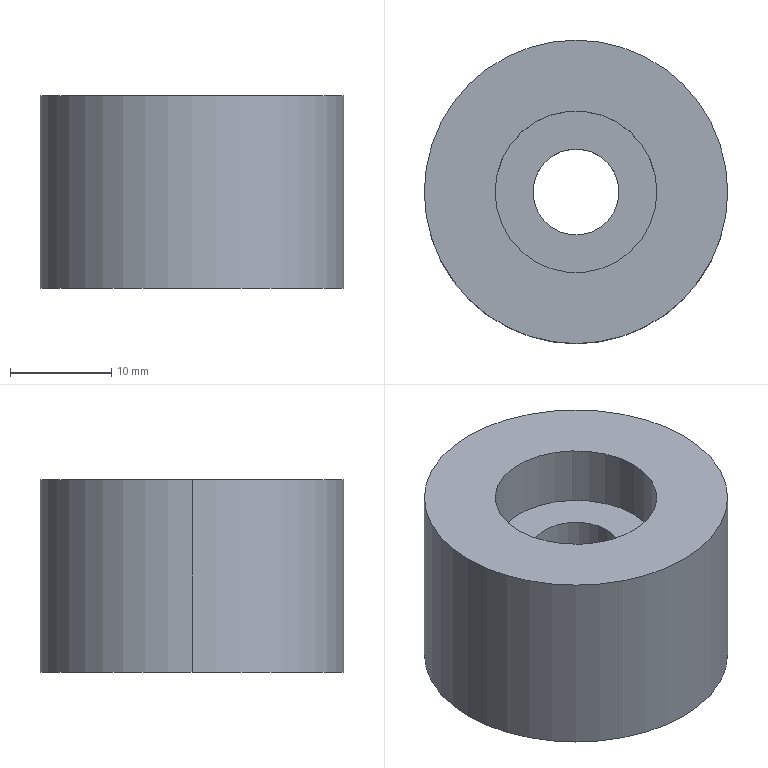Part | STEP file | POM limit 1 | 1 solid | 9 faces | box 30 x 30 x 19 mm | volume 11486 mm3 | cylinder 6 | plane 3 | commonest cylinder face diameters 8.5 x2 16 x2 30 x2
STEP:
#1=CARTESIAN_POINT('',(0.,0.,0.));
#2=DIRECTION('',(0.,0.,1.));
#3=DIRECTION('',(1.,0.,0.));
#4=AXIS2_PLACEMENT_3D('',#1,#2,#3);
#5=CARTESIAN_POINT('',(8.,0.,13.));
#6=VERTEX_POINT('',#5);
#7=CARTESIAN_POINT('',(8.,0.,19.));
#8=VERTEX_POINT('',#7);
#9=CARTESIAN_POINT('',(8.,0.,13.));
#10=DIRECTION('',(0.,0.,1.));
#11=VECTOR('',#10,1.);
#12=LINE('',#9,#11);
#13=CARTESIAN_POINT('',(0.,0.,13.));
#14=DIRECTION('',(0.,0.,1.));
#15=DIRECTION('',(1.,0.,0.));
#16=AXIS2_PLACEMENT_3D('',#13,#14,#15);
#17=CYLINDRICAL_SURFACE('',#16,8.);
#18=CARTESIAN_POINT('',(6.283,0.));
#19=DIRECTION('',(0.,1.));
#20=VECTOR('',#19,1.);
#21=LINE('',#18,#20);
#22=(GEOMETRIC_REPRESENTATION_CONTEXT(2)PARAMETRIC_REPRESENTATION_CONTEXT()REPRESENTATION_CONTEXT('',''));
#23=DEFINITIONAL_REPRESENTATION('',(#21),#22);
#24=PCURVE('',#17,#23);
#25=CARTESIAN_POINT('',(0.,0.,13.));
#26=DIRECTION('',(0.,0.,1.));
#27=DIRECTION('',(1.,0.,0.));
#28=AXIS2_PLACEMENT_3D('',#25,#26,#27);
#29=CYLINDRICAL_SURFACE('',#28,8.);
#30=CARTESIAN_POINT('',(0.,0.));
#31=DIRECTION('',(0.,1.));
#32=VECTOR('',#31,1.);
#33=LINE('',#30,#32);
#34=(GEOMETRIC_REPRESENTATION_CONTEXT(2)PARAMETRIC_REPRESENTATION_CONTEXT()REPRESENTATION_CONTEXT('',''));
#35=DEFINITIONAL_REPRESENTATION('',(#33),#34);
#36=PCURVE('',#29,#35);
#37=SURFACE_CURVE('',#12,(#24,#36),.PCURVE_S1.);
#38=EDGE_CURVE('',#6,#8,#37,.T.);
#39=ORIENTED_EDGE('',*,*,#38,.T.);
#40=CARTESIAN_POINT('',(-8.,0.,19.));
#41=VERTEX_POINT('',#40);
#42=CARTESIAN_POINT('',(0.,0.,19.));
#43=DIRECTION('',(0.,0.,1.));
#44=DIRECTION('',(1.,0.,0.));
#45=AXIS2_PLACEMENT_3D('',#42,#43,#44);
#46=CIRCLE('',#45,8.);
#47=CARTESIAN_POINT('',(0.,6.));
#48=DIRECTION('',(1.,0.));
#49=VECTOR('',#48,1.);
#50=LINE('',#47,#49);
#51=(GEOMETRIC_REPRESENTATION_CONTEXT(2)PARAMETRIC_REPRESENTATION_CONTEXT()REPRESENTATION_CONTEXT('',''));
#52=DEFINITIONAL_REPRESENTATION('',(#50),#51);
#53=PCURVE('',#17,#52);
#54=CARTESIAN_POINT('',(0.,0.,19.));
#55=DIRECTION('',(0.,0.,1.));
#56=DIRECTION('',(1.,0.,0.));
#57=AXIS2_PLACEMENT_3D('',#54,#55,#56);
#58=PLANE('',#57);
#59=CARTESIAN_POINT('',(0.,0.));
#60=DIRECTION('',(1.,0.));
#61=AXIS2_PLACEMENT_2D('',#59,#60);
#62=CIRCLE('',#61,8.);
#63=(GEOMETRIC_REPRESENTATION_CONTEXT(2)PARAMETRIC_REPRESENTATION_CONTEXT()REPRESENTATION_CONTEXT('',''));
#64=DEFINITIONAL_REPRESENTATION('',(#62),#63);
#65=PCURVE('',#58,#64);
#66=SURFACE_CURVE('',#46,(#53,#65),.PCURVE_S1.);
#67=EDGE_CURVE('',#41,#8,#66,.T.);
#68=ORIENTED_EDGE('',*,*,#67,.F.);
#69=CARTESIAN_POINT('',(-8.,0.,13.));
#70=VERTEX_POINT('',#69);
#71=CARTESIAN_POINT('',(-8.,0.,13.));
#72=DIRECTION('',(0.,0.,1.));
#73=VECTOR('',#72,1.);
#74=LINE('',#71,#73);
#75=CARTESIAN_POINT('',(3.142,0.));
#76=DIRECTION('',(0.,1.));
#77=VECTOR('',#76,1.);
#78=LINE('',#75,#77);
#79=(GEOMETRIC_REPRESENTATION_CONTEXT(2)PARAMETRIC_REPRESENTATION_CONTEXT()REPRESENTATION_CONTEXT('',''));
#80=DEFINITIONAL_REPRESENTATION('',(#78),#79);
#81=PCURVE('',#17,#80);
#82=CARTESIAN_POINT('',(3.142,0.));
#83=DIRECTION('',(0.,1.));
#84=VECTOR('',#83,1.);
#85=LINE('',#82,#84);
#86=(GEOMETRIC_REPRESENTATION_CONTEXT(2)PARAMETRIC_REPRESENTATION_CONTEXT()REPRESENTATION_CONTEXT('',''));
#87=DEFINITIONAL_REPRESENTATION('',(#85),#86);
#88=PCURVE('',#29,#87);
#89=SURFACE_CURVE('',#74,(#81,#88),.PCURVE_S1.);
#90=EDGE_CURVE('',#70,#41,#89,.T.);
#91=ORIENTED_EDGE('',*,*,#90,.F.);
#92=CARTESIAN_POINT('',(0.,0.,13.));
#93=DIRECTION('',(0.,0.,1.));
#94=DIRECTION('',(1.,0.,0.));
#95=AXIS2_PLACEMENT_3D('',#92,#93,#94);
#96=CIRCLE('',#95,8.);
#97=CARTESIAN_POINT('',(0.,0.));
#98=DIRECTION('',(1.,0.));
#99=VECTOR('',#98,1.);
#100=LINE('',#97,#99);
#101=(GEOMETRIC_REPRESENTATION_CONTEXT(2)PARAMETRIC_REPRESENTATION_CONTEXT()REPRESENTATION_CONTEXT('',''));
#102=DEFINITIONAL_REPRESENTATION('',(#100),#101);
#103=PCURVE('',#17,#102);
#104=CARTESIAN_POINT('',(0.,0.,13.));
#105=DIRECTION('',(0.,0.,1.));
#106=DIRECTION('',(1.,0.,0.));
#107=AXIS2_PLACEMENT_3D('',#104,#105,#106);
#108=PLANE('',#107);
#109=CARTESIAN_POINT('',(0.,0.));
#110=DIRECTION('',(1.,0.));
#111=AXIS2_PLACEMENT_2D('',#109,#110);
#112=CIRCLE('',#111,8.);
#113=(GEOMETRIC_REPRESENTATION_CONTEXT(2)PARAMETRIC_REPRESENTATION_CONTEXT()REPRESENTATION_CONTEXT('',''));
#114=DEFINITIONAL_REPRESENTATION('',(#112),#113);
#115=PCURVE('',#108,#114);
#116=SURFACE_CURVE('',#96,(#103,#115),.PCURVE_S1.);
#117=EDGE_CURVE('',#70,#6,#116,.T.);
#118=ORIENTED_EDGE('',*,*,#117,.T.);
#119=EDGE_LOOP('',(#39,#68,#91,#118));
#120=FACE_BOUND('',#119,.F.);
#121=ADVANCED_FACE('',(#120),#17,.F.);
#122=CARTESIAN_POINT('',(15.,0.,19.));
#123=VERTEX_POINT('',#122);
#124=CARTESIAN_POINT('',(-15.,0.,19.));
#125=VERTEX_POINT('',#124);
#126=CARTESIAN_POINT('',(0.,0.,19.));
#127=DIRECTION('',(0.,0.,1.));
#128=DIRECTION('',(1.,0.,0.));
#129=AXIS2_PLACEMENT_3D('',#126,#127,#128);
#130=CIRCLE('',#129,15.);
#131=CARTESIAN_POINT('',(0.,0.,19.));
#132=DIRECTION('',(0.,0.,-1.));
#133=DIRECTION('',(-1.,0.,0.));
#134=AXIS2_PLACEMENT_3D('',#131,#132,#133);
#135=CYLINDRICAL_SURFACE('',#134,15.);
#136=CARTESIAN_POINT('',(3.142,0.));
#137=DIRECTION('',(-1.,0.));
#138=VECTOR('',#137,1.);
#139=LINE('',#136,#138);
#140=(GEOMETRIC_REPRESENTATION_CONTEXT(2)PARAMETRIC_REPRESENTATION_CONTEXT()REPRESENTATION_CONTEXT('',''));
#141=DEFINITIONAL_REPRESENTATION('',(#139),#140);
#142=PCURVE('',#135,#141);
#143=CARTESIAN_POINT('',(0.,0.));
#144=DIRECTION('',(1.,0.));
#145=AXIS2_PLACEMENT_2D('',#143,#144);
#146=CIRCLE('',#145,15.);
#147=(GEOMETRIC_REPRESENTATION_CONTEXT(2)PARAMETRIC_REPRESENTATION_CONTEXT()REPRESENTATION_CONTEXT('',''));
#148=DEFINITIONAL_REPRESENTATION('',(#146),#147);
#149=PCURVE('',#58,#148);
#150=SURFACE_CURVE('',#130,(#142,#149),.PCURVE_S1.);
#151=EDGE_CURVE('',#123,#125,#150,.T.);
#152=ORIENTED_EDGE('',*,*,#151,.F.);
#153=CARTESIAN_POINT('',(15.,0.,0.));
#154=VERTEX_POINT('',#153);
#155=CARTESIAN_POINT('',(15.,0.,19.));
#156=DIRECTION('',(0.,0.,-1.));
#157=VECTOR('',#156,1.);
#158=LINE('',#155,#157);
#159=CARTESIAN_POINT('',(3.142,0.));
#160=DIRECTION('',(0.,1.));
#161=VECTOR('',#160,1.);
#162=LINE('',#159,#161);
#163=(GEOMETRIC_REPRESENTATION_CONTEXT(2)PARAMETRIC_REPRESENTATION_CONTEXT()REPRESENTATION_CONTEXT('',''));
#164=DEFINITIONAL_REPRESENTATION('',(#162),#163);
#165=PCURVE('',#135,#164);
#166=CARTESIAN_POINT('',(0.,0.,19.));
#167=DIRECTION('',(0.,0.,-1.));
#168=DIRECTION('',(-1.,0.,0.));
#169=AXIS2_PLACEMENT_3D('',#166,#167,#168);
#170=CYLINDRICAL_SURFACE('',#169,15.);
#171=CARTESIAN_POINT('',(3.142,0.));
#172=DIRECTION('',(0.,1.));
#173=VECTOR('',#172,1.);
#174=LINE('',#171,#173);
#175=(GEOMETRIC_REPRESENTATION_CONTEXT(2)PARAMETRIC_REPRESENTATION_CONTEXT()REPRESENTATION_CONTEXT('',''));
#176=DEFINITIONAL_REPRESENTATION('',(#174),#175);
#177=PCURVE('',#170,#176);
#178=SURFACE_CURVE('',#158,(#165,#177),.PCURVE_S1.);
#179=EDGE_CURVE('',#123,#154,#178,.T.);
#180=ORIENTED_EDGE('',*,*,#179,.T.);
#181=CARTESIAN_POINT('',(-15.,0.,0.));
#182=VERTEX_POINT('',#181);
#183=CARTESIAN_POINT('',(0.,0.,0.));
#184=DIRECTION('',(0.,0.,1.));
#185=DIRECTION('',(1.,0.,0.));
#186=AXIS2_PLACEMENT_3D('',#183,#184,#185);
#187=CIRCLE('',#186,15.);
#188=CARTESIAN_POINT('',(3.142,19.));
#189=DIRECTION('',(-1.,0.));
#190=VECTOR('',#189,1.);
#191=LINE('',#188,#190);
#192=(GEOMETRIC_REPRESENTATION_CONTEXT(2)PARAMETRIC_REPRESENTATION_CONTEXT()REPRESENTATION_CONTEXT('',''));
#193=DEFINITIONAL_REPRESENTATION('',(#191),#192);
#194=PCURVE('',#135,#193);
#195=CARTESIAN_POINT('',(0.,0.,0.));
#196=DIRECTION('',(0.,0.,1.));
#197=DIRECTION('',(1.,0.,0.));
#198=AXIS2_PLACEMENT_3D('',#195,#196,#197);
#199=PLANE('',#198);
#200=CARTESIAN_POINT('',(0.,0.));
#201=DIRECTION('',(1.,0.));
#202=AXIS2_PLACEMENT_2D('',#200,#201);
#203=CIRCLE('',#202,15.);
#204=(GEOMETRIC_REPRESENTATION_CONTEXT(2)PARAMETRIC_REPRESENTATION_CONTEXT()REPRESENTATION_CONTEXT('',''));
#205=DEFINITIONAL_REPRESENTATION('',(#203),#204);
#206=PCURVE('',#199,#205);
#207=SURFACE_CURVE('',#187,(#194,#206),.PCURVE_S1.);
#208=EDGE_CURVE('',#154,#182,#207,.T.);
#209=ORIENTED_EDGE('',*,*,#208,.T.);
#210=CARTESIAN_POINT('',(-15.,0.,19.));
#211=DIRECTION('',(0.,0.,-1.));
#212=VECTOR('',#211,1.);
#213=LINE('',#210,#212);
#214=CARTESIAN_POINT('',(0.,0.));
#215=DIRECTION('',(0.,1.));
#216=VECTOR('',#215,1.);
#217=LINE('',#214,#216);
#218=(GEOMETRIC_REPRESENTATION_CONTEXT(2)PARAMETRIC_REPRESENTATION_CONTEXT()REPRESENTATION_CONTEXT('',''));
#219=DEFINITIONAL_REPRESENTATION('',(#217),#218);
#220=PCURVE('',#135,#219);
#221=CARTESIAN_POINT('',(6.283,0.));
#222=DIRECTION('',(0.,1.));
#223=VECTOR('',#222,1.);
#224=LINE('',#221,#223);
#225=(GEOMETRIC_REPRESENTATION_CONTEXT(2)PARAMETRIC_REPRESENTATION_CONTEXT()REPRESENTATION_CONTEXT('',''));
#226=DEFINITIONAL_REPRESENTATION('',(#224),#225);
#227=PCURVE('',#170,#226);
#228=SURFACE_CURVE('',#213,(#220,#227),.PCURVE_S1.);
#229=EDGE_CURVE('',#125,#182,#228,.T.);
#230=ORIENTED_EDGE('',*,*,#229,.F.);
#231=EDGE_LOOP('',(#152,#180,#209,#230));
#232=FACE_BOUND('',#231,.T.);
#233=ADVANCED_FACE('',(#232),#135,.T.);
#234=CARTESIAN_POINT('',(-4.25,0.,13.));
#235=VERTEX_POINT('',#234);
#236=CARTESIAN_POINT('',(-4.25,0.,0.));
#237=VERTEX_POINT('',#236);
#238=CARTESIAN_POINT('',(-4.25,0.,19.));
#239=DIRECTION('',(0.,0.,-1.));
#240=VECTOR('',#239,1.);
#241=LINE('',#238,#240);
#242=CARTESIAN_POINT('',(0.,0.,19.));
#243=DIRECTION('',(0.,0.,-1.));
#244=DIRECTION('',(-1.,0.,0.));
#245=AXIS2_PLACEMENT_3D('',#242,#243,#244);
#246=CYLINDRICAL_SURFACE('',#245,4.25);
#247=CARTESIAN_POINT('',(6.283,0.));
#248=DIRECTION('',(0.,1.));
#249=VECTOR('',#248,1.);
#250=LINE('',#247,#249);
#251=(GEOMETRIC_REPRESENTATION_CONTEXT(2)PARAMETRIC_REPRESENTATION_CONTEXT()REPRESENTATION_CONTEXT('',''));
#252=DEFINITIONAL_REPRESENTATION('',(#250),#251);
#253=PCURVE('',#246,#252);
#254=CARTESIAN_POINT('',(0.,0.,19.));
#255=DIRECTION('',(0.,0.,-1.));
#256=DIRECTION('',(-1.,0.,0.));
#257=AXIS2_PLACEMENT_3D('',#254,#255,#256);
#258=CYLINDRICAL_SURFACE('',#257,4.25);
#259=CARTESIAN_POINT('',(0.,0.));
#260=DIRECTION('',(0.,1.));
#261=VECTOR('',#260,1.);
#262=LINE('',#259,#261);
#263=(GEOMETRIC_REPRESENTATION_CONTEXT(2)PARAMETRIC_REPRESENTATION_CONTEXT()REPRESENTATION_CONTEXT('',''));
#264=DEFINITIONAL_REPRESENTATION('',(#262),#263);
#265=PCURVE('',#258,#264);
#266=SURFACE_CURVE('',#241,(#253,#265),.PCURVE_S1.);
#267=EDGE_CURVE('',#235,#237,#266,.T.);
#268=ORIENTED_EDGE('',*,*,#267,.T.);
#269=CARTESIAN_POINT('',(4.25,0.,0.));
#270=VERTEX_POINT('',#269);
#271=CARTESIAN_POINT('',(0.,0.,0.));
#272=DIRECTION('',(0.,0.,1.));
#273=DIRECTION('',(1.,0.,0.));
#274=AXIS2_PLACEMENT_3D('',#271,#272,#273);
#275=CIRCLE('',#274,4.25);
#276=CARTESIAN_POINT('',(9.425,19.));
#277=DIRECTION('',(-1.,0.));
#278=VECTOR('',#277,1.);
#279=LINE('',#276,#278);
#280=(GEOMETRIC_REPRESENTATION_CONTEXT(2)PARAMETRIC_REPRESENTATION_CONTEXT()REPRESENTATION_CONTEXT('',''));
#281=DEFINITIONAL_REPRESENTATION('',(#279),#280);
#282=PCURVE('',#246,#281);
#283=CARTESIAN_POINT('',(0.,0.));
#284=DIRECTION('',(1.,0.));
#285=AXIS2_PLACEMENT_2D('',#283,#284);
#286=CIRCLE('',#285,4.25);
#287=(GEOMETRIC_REPRESENTATION_CONTEXT(2)PARAMETRIC_REPRESENTATION_CONTEXT()REPRESENTATION_CONTEXT('',''));
#288=DEFINITIONAL_REPRESENTATION('',(#286),#287);
#289=PCURVE('',#199,#288);
#290=SURFACE_CURVE('',#275,(#282,#289),.PCURVE_S1.);
#291=EDGE_CURVE('',#237,#270,#290,.T.);
#292=ORIENTED_EDGE('',*,*,#291,.T.);
#293=CARTESIAN_POINT('',(4.25,0.,13.));
#294=VERTEX_POINT('',#293);
#295=CARTESIAN_POINT('',(4.25,0.,19.));
#296=DIRECTION('',(0.,0.,-1.));
#297=VECTOR('',#296,1.);
#298=LINE('',#295,#297);
#299=CARTESIAN_POINT('',(3.142,0.));
#300=DIRECTION('',(0.,1.));
#301=VECTOR('',#300,1.);
#302=LINE('',#299,#301);
#303=(GEOMETRIC_REPRESENTATION_CONTEXT(2)PARAMETRIC_REPRESENTATION_CONTEXT()REPRESENTATION_CONTEXT('',''));
#304=DEFINITIONAL_REPRESENTATION('',(#302),#303);
#305=PCURVE('',#246,#304);
#306=CARTESIAN_POINT('',(3.142,0.));
#307=DIRECTION('',(0.,1.));
#308=VECTOR('',#307,1.);
#309=LINE('',#306,#308);
#310=(GEOMETRIC_REPRESENTATION_CONTEXT(2)PARAMETRIC_REPRESENTATION_CONTEXT()REPRESENTATION_CONTEXT('',''));
#311=DEFINITIONAL_REPRESENTATION('',(#309),#310);
#312=PCURVE('',#258,#311);
#313=SURFACE_CURVE('',#298,(#305,#312),.PCURVE_S1.);
#314=EDGE_CURVE('',#294,#270,#313,.T.);
#315=ORIENTED_EDGE('',*,*,#314,.F.);
#316=CARTESIAN_POINT('',(0.,0.,13.));
#317=DIRECTION('',(0.,0.,1.));
#318=DIRECTION('',(1.,0.,0.));
#319=AXIS2_PLACEMENT_3D('',#316,#317,#318);
#320=CIRCLE('',#319,4.25);
#321=CARTESIAN_POINT('',(9.425,6.));
#322=DIRECTION('',(-1.,0.));
#323=VECTOR('',#322,1.);
#324=LINE('',#321,#323);
#325=(GEOMETRIC_REPRESENTATION_CONTEXT(2)PARAMETRIC_REPRESENTATION_CONTEXT()REPRESENTATION_CONTEXT('',''));
#326=DEFINITIONAL_REPRESENTATION('',(#324),#325);
#327=PCURVE('',#246,#326);
#328=CARTESIAN_POINT('',(0.,0.));
#329=DIRECTION('',(1.,0.));
#330=AXIS2_PLACEMENT_2D('',#328,#329);
#331=CIRCLE('',#330,4.25);
#332=(GEOMETRIC_REPRESENTATION_CONTEXT(2)PARAMETRIC_REPRESENTATION_CONTEXT()REPRESENTATION_CONTEXT('',''));
#333=DEFINITIONAL_REPRESENTATION('',(#331),#332);
#334=PCURVE('',#108,#333);
#335=SURFACE_CURVE('',#320,(#327,#334),.PCURVE_S1.);
#336=EDGE_CURVE('',#235,#294,#335,.T.);
#337=ORIENTED_EDGE('',*,*,#336,.F.);
#338=EDGE_LOOP('',(#268,#292,#315,#337));
#339=FACE_BOUND('',#338,.F.);
#340=ADVANCED_FACE('',(#339),#246,.F.);
#341=CARTESIAN_POINT('',(0.,0.,0.));
#342=DIRECTION('',(0.,0.,1.));
#343=DIRECTION('',(1.,0.,0.));
#344=AXIS2_PLACEMENT_3D('',#341,#342,#343);
#345=CIRCLE('',#344,4.25);
#346=CARTESIAN_POINT('',(3.142,19.));
#347=DIRECTION('',(-1.,0.));
#348=VECTOR('',#347,1.);
#349=LINE('',#346,#348);
#350=(GEOMETRIC_REPRESENTATION_CONTEXT(2)PARAMETRIC_REPRESENTATION_CONTEXT()REPRESENTATION_CONTEXT('',''));
#351=DEFINITIONAL_REPRESENTATION('',(#349),#350);
#352=PCURVE('',#258,#351);
#353=CARTESIAN_POINT('',(0.,0.));
#354=DIRECTION('',(1.,0.));
#355=AXIS2_PLACEMENT_2D('',#353,#354);
#356=CIRCLE('',#355,4.25);
#357=(GEOMETRIC_REPRESENTATION_CONTEXT(2)PARAMETRIC_REPRESENTATION_CONTEXT()REPRESENTATION_CONTEXT('',''));
#358=DEFINITIONAL_REPRESENTATION('',(#356),#357);
#359=PCURVE('',#199,#358);
#360=SURFACE_CURVE('',#345,(#352,#359),.PCURVE_S1.);
#361=EDGE_CURVE('',#270,#237,#360,.T.);
#362=ORIENTED_EDGE('',*,*,#361,.T.);
#363=ORIENTED_EDGE('',*,*,#267,.F.);
#364=CARTESIAN_POINT('',(0.,0.,13.));
#365=DIRECTION('',(0.,0.,1.));
#366=DIRECTION('',(1.,0.,0.));
#367=AXIS2_PLACEMENT_3D('',#364,#365,#366);
#368=CIRCLE('',#367,4.25);
#369=CARTESIAN_POINT('',(3.142,6.));
#370=DIRECTION('',(-1.,0.));
#371=VECTOR('',#370,1.);
#372=LINE('',#369,#371);
#373=(GEOMETRIC_REPRESENTATION_CONTEXT(2)PARAMETRIC_REPRESENTATION_CONTEXT()REPRESENTATION_CONTEXT('',''));
#374=DEFINITIONAL_REPRESENTATION('',(#372),#373);
#375=PCURVE('',#258,#374);
#376=CARTESIAN_POINT('',(0.,0.));
#377=DIRECTION('',(1.,0.));
#378=AXIS2_PLACEMENT_2D('',#376,#377);
#379=CIRCLE('',#378,4.25);
#380=(GEOMETRIC_REPRESENTATION_CONTEXT(2)PARAMETRIC_REPRESENTATION_CONTEXT()REPRESENTATION_CONTEXT('',''));
#381=DEFINITIONAL_REPRESENTATION('',(#379),#380);
#382=PCURVE('',#108,#381);
#383=SURFACE_CURVE('',#368,(#375,#382),.PCURVE_S1.);
#384=EDGE_CURVE('',#294,#235,#383,.T.);
#385=ORIENTED_EDGE('',*,*,#384,.F.);
#386=ORIENTED_EDGE('',*,*,#314,.T.);
#387=EDGE_LOOP('',(#362,#363,#385,#386));
#388=FACE_BOUND('',#387,.F.);
#389=ADVANCED_FACE('',(#388),#258,.F.);
#390=CARTESIAN_POINT('',(0.,0.,19.));
#391=DIRECTION('',(0.,0.,1.));
#392=DIRECTION('',(1.,0.,0.));
#393=AXIS2_PLACEMENT_3D('',#390,#391,#392);
#394=CIRCLE('',#393,8.);
#395=CARTESIAN_POINT('',(0.,0.));
#396=DIRECTION('',(1.,0.));
#397=AXIS2_PLACEMENT_2D('',#395,#396);
#398=CIRCLE('',#397,8.);
#399=(GEOMETRIC_REPRESENTATION_CONTEXT(2)PARAMETRIC_REPRESENTATION_CONTEXT()REPRESENTATION_CONTEXT('',''));
#400=DEFINITIONAL_REPRESENTATION('',(#398),#399);
#401=PCURVE('',#58,#400);
#402=CARTESIAN_POINT('',(0.,6.));
#403=DIRECTION('',(1.,0.));
#404=VECTOR('',#403,1.);
#405=LINE('',#402,#404);
#406=(GEOMETRIC_REPRESENTATION_CONTEXT(2)PARAMETRIC_REPRESENTATION_CONTEXT()REPRESENTATION_CONTEXT('',''));
#407=DEFINITIONAL_REPRESENTATION('',(#405),#406);
#408=PCURVE('',#29,#407);
#409=SURFACE_CURVE('',#394,(#401,#408),.PCURVE_S1.);
#410=EDGE_CURVE('',#8,#41,#409,.T.);
#411=ORIENTED_EDGE('',*,*,#410,.F.);
#412=ORIENTED_EDGE('',*,*,#67,.F.);
#413=EDGE_LOOP('',(#411,#412));
#414=FACE_BOUND('',#413,.T.);
#415=CARTESIAN_POINT('',(0.,0.,19.));
#416=DIRECTION('',(0.,0.,1.));
#417=DIRECTION('',(1.,0.,0.));
#418=AXIS2_PLACEMENT_3D('',#415,#416,#417);
#419=CIRCLE('',#418,15.);
#420=CARTESIAN_POINT('',(0.,0.));
#421=DIRECTION('',(1.,0.));
#422=AXIS2_PLACEMENT_2D('',#420,#421);
#423=CIRCLE('',#422,15.);
#424=(GEOMETRIC_REPRESENTATION_CONTEXT(2)PARAMETRIC_REPRESENTATION_CONTEXT()REPRESENTATION_CONTEXT('',''));
#425=DEFINITIONAL_REPRESENTATION('',(#423),#424);
#426=PCURVE('',#58,#425);
#427=CARTESIAN_POINT('',(9.425,0.));
#428=DIRECTION('',(-1.,0.));
#429=VECTOR('',#428,1.);
#430=LINE('',#427,#429);
#431=(GEOMETRIC_REPRESENTATION_CONTEXT(2)PARAMETRIC_REPRESENTATION_CONTEXT()REPRESENTATION_CONTEXT('',''));
#432=DEFINITIONAL_REPRESENTATION('',(#430),#431);
#433=PCURVE('',#170,#432);
#434=SURFACE_CURVE('',#419,(#426,#433),.PCURVE_S1.);
#435=EDGE_CURVE('',#125,#123,#434,.T.);
#436=ORIENTED_EDGE('',*,*,#435,.T.);
#437=ORIENTED_EDGE('',*,*,#151,.T.);
#438=EDGE_LOOP('',(#436,#437));
#439=FACE_BOUND('',#438,.T.);
#440=ADVANCED_FACE('',(#414,#439),#58,.T.);
#441=CARTESIAN_POINT('',(0.,0.,0.));
#442=DIRECTION('',(0.,0.,1.));
#443=DIRECTION('',(1.,0.,0.));
#444=AXIS2_PLACEMENT_3D('',#441,#442,#443);
#445=CIRCLE('',#444,15.);
#446=CARTESIAN_POINT('',(0.,0.));
#447=DIRECTION('',(1.,0.));
#448=AXIS2_PLACEMENT_2D('',#446,#447);
#449=CIRCLE('',#448,15.);
#450=(GEOMETRIC_REPRESENTATION_CONTEXT(2)PARAMETRIC_REPRESENTATION_CONTEXT()REPRESENTATION_CONTEXT('',''));
#451=DEFINITIONAL_REPRESENTATION('',(#449),#450);
#452=PCURVE('',#199,#451);
#453=CARTESIAN_POINT('',(9.425,19.));
#454=DIRECTION('',(-1.,0.));
#455=VECTOR('',#454,1.);
#456=LINE('',#453,#455);
#457=(GEOMETRIC_REPRESENTATION_CONTEXT(2)PARAMETRIC_REPRESENTATION_CONTEXT()REPRESENTATION_CONTEXT('',''));
#458=DEFINITIONAL_REPRESENTATION('',(#456),#457);
#459=PCURVE('',#170,#458);
#460=SURFACE_CURVE('',#445,(#452,#459),.PCURVE_S1.);
#461=EDGE_CURVE('',#182,#154,#460,.T.);
#462=ORIENTED_EDGE('',*,*,#461,.F.);
#463=ORIENTED_EDGE('',*,*,#208,.F.);
#464=EDGE_LOOP('',(#462,#463));
#465=FACE_BOUND('',#464,.T.);
#466=ORIENTED_EDGE('',*,*,#291,.T.);
#467=ORIENTED_EDGE('',*,*,#361,.T.);
#468=EDGE_LOOP('',(#466,#467));
#469=FACE_BOUND('',#468,.T.);
#470=ADVANCED_FACE('',(#465,#469),#199,.F.);
#471=ORIENTED_EDGE('',*,*,#179,.F.);
#472=ORIENTED_EDGE('',*,*,#435,.F.);
#473=ORIENTED_EDGE('',*,*,#229,.T.);
#474=ORIENTED_EDGE('',*,*,#461,.T.);
#475=EDGE_LOOP('',(#471,#472,#473,#474));
#476=FACE_BOUND('',#475,.T.);
#477=ADVANCED_FACE('',(#476),#170,.T.);
#478=ORIENTED_EDGE('',*,*,#410,.F.);
#479=ORIENTED_EDGE('',*,*,#38,.F.);
#480=CARTESIAN_POINT('',(0.,0.,13.));
#481=DIRECTION('',(0.,0.,1.));
#482=DIRECTION('',(1.,0.,0.));
#483=AXIS2_PLACEMENT_3D('',#480,#481,#482);
#484=CIRCLE('',#483,8.);
#485=CARTESIAN_POINT('',(0.,0.));
#486=DIRECTION('',(1.,0.));
#487=VECTOR('',#486,1.);
#488=LINE('',#485,#487);
#489=(GEOMETRIC_REPRESENTATION_CONTEXT(2)PARAMETRIC_REPRESENTATION_CONTEXT()REPRESENTATION_CONTEXT('',''));
#490=DEFINITIONAL_REPRESENTATION('',(#488),#489);
#491=PCURVE('',#29,#490);
#492=CARTESIAN_POINT('',(0.,0.));
#493=DIRECTION('',(1.,0.));
#494=AXIS2_PLACEMENT_2D('',#492,#493);
#495=CIRCLE('',#494,8.);
#496=(GEOMETRIC_REPRESENTATION_CONTEXT(2)PARAMETRIC_REPRESENTATION_CONTEXT()REPRESENTATION_CONTEXT('',''));
#497=DEFINITIONAL_REPRESENTATION('',(#495),#496);
#498=PCURVE('',#108,#497);
#499=SURFACE_CURVE('',#484,(#491,#498),.PCURVE_S1.);
#500=EDGE_CURVE('',#6,#70,#499,.T.);
#501=ORIENTED_EDGE('',*,*,#500,.T.);
#502=ORIENTED_EDGE('',*,*,#90,.T.);
#503=EDGE_LOOP('',(#478,#479,#501,#502));
#504=FACE_BOUND('',#503,.F.);
#505=ADVANCED_FACE('',(#504),#29,.F.);
#506=ORIENTED_EDGE('',*,*,#336,.F.);
#507=ORIENTED_EDGE('',*,*,#384,.F.);
#508=EDGE_LOOP('',(#506,#507));
#509=FACE_BOUND('',#508,.T.);
#510=ORIENTED_EDGE('',*,*,#500,.T.);
#511=ORIENTED_EDGE('',*,*,#117,.T.);
#512=EDGE_LOOP('',(#510,#511));
#513=FACE_BOUND('',#512,.T.);
#514=ADVANCED_FACE('',(#509,#513),#108,.T.);
#515=CLOSED_SHELL('',(#121,#233,#340,#389,#440,#470,#477,#505,#514));
#516=MANIFOLD_SOLID_BREP('',#515);
#517=(LENGTH_UNIT()NAMED_UNIT(*)SI_UNIT(.MILLI.,.METRE.));
#518=UNCERTAINTY_MEASURE_WITH_UNIT(LENGTH_MEASURE(0.0000001),#517,'','');
#519=(NAMED_UNIT(*)PLANE_ANGLE_UNIT()SI_UNIT($,.RADIAN.));
#520=(NAMED_UNIT(*)SI_UNIT($,.STERADIAN.)SOLID_ANGLE_UNIT());
#521=(GEOMETRIC_REPRESENTATION_CONTEXT(3)GLOBAL_UNCERTAINTY_ASSIGNED_CONTEXT((#518))GLOBAL_UNIT_ASSIGNED_CONTEXT((#517,#519,#520))REPRESENTATION_CONTEXT('',''));
#522=ADVANCED_BREP_SHAPE_REPRESENTATION('',(#4,#516),#521);